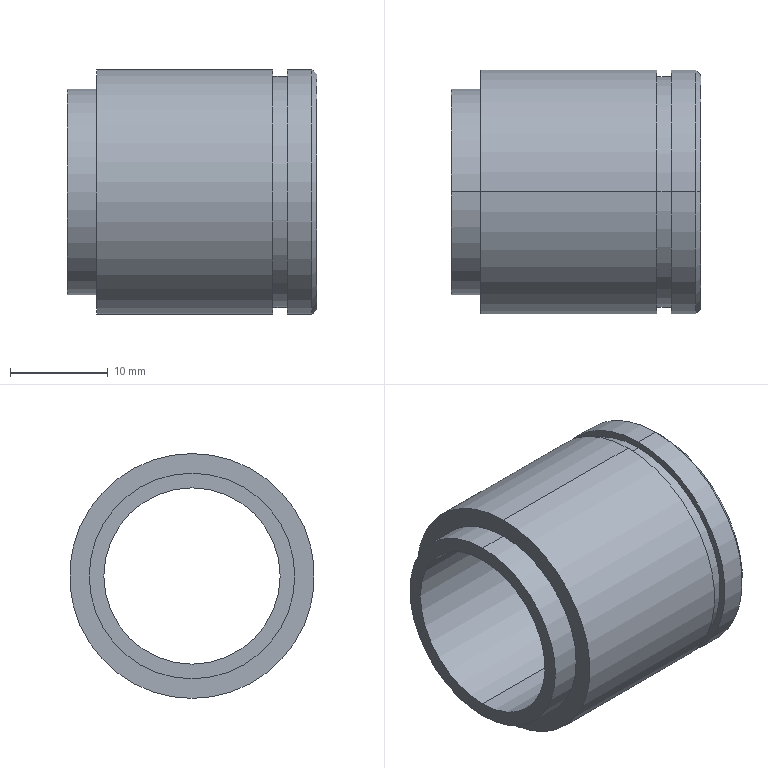Part | STEP file | 1 solid | 19 faces | box 25.5 x 25 x 25 mm | volume 5476 mm3 | cylinder 10 | plane 5 | cone 4 | commonest cylinder face diameters 25 x4 18 x2 21 x2 23.6 x2
STEP:
#1=CARTESIAN_POINT('',(0.,0.,0.));
#2=DIRECTION('',(0.,0.,1.));
#3=DIRECTION('',(1.,0.,0.));
#4=AXIS2_PLACEMENT_3D('',#1,#2,#3);
#5=CARTESIAN_POINT('',(3.,0.,-12.5));
#6=VERTEX_POINT('',#5);
#7=CARTESIAN_POINT('',(3.,0.,12.5));
#8=VERTEX_POINT('',#7);
#9=CARTESIAN_POINT('',(3.,0.,0.));
#10=DIRECTION('',(1.,0.,0.));
#11=DIRECTION('',(0.,0.,-1.));
#12=AXIS2_PLACEMENT_3D('',#9,#10,#11);
#13=CIRCLE('',#12,12.5);
#14=CARTESIAN_POINT('',(12.,0.,0.));
#15=DIRECTION('',(1.,0.,0.));
#16=DIRECTION('',(0.,0.,-1.));
#17=AXIS2_PLACEMENT_3D('',#14,#15,#16);
#18=CYLINDRICAL_SURFACE('',#17,12.5);
#19=CARTESIAN_POINT('',(0.,-9.));
#20=DIRECTION('',(1.,0.));
#21=VECTOR('',#20,1.);
#22=LINE('',#19,#21);
#23=(GEOMETRIC_REPRESENTATION_CONTEXT(2)PARAMETRIC_REPRESENTATION_CONTEXT()REPRESENTATION_CONTEXT('',''));
#24=DEFINITIONAL_REPRESENTATION('',(#22),#23);
#25=PCURVE('',#18,#24);
#26=CARTESIAN_POINT('',(3.,11.5,0.));
#27=DIRECTION('',(-1.,0.,0.));
#28=DIRECTION('',(0.,0.,1.));
#29=AXIS2_PLACEMENT_3D('',#26,#27,#28);
#30=PLANE('',#29);
#31=CARTESIAN_POINT('',(-12.5,-11.5));
#32=CARTESIAN_POINT('',(-12.5,10.151));
#33=CARTESIAN_POINT('',(6.25,-0.6747));
#34=CARTESIAN_POINT('',(25.,-11.5));
#35=CARTESIAN_POINT('',(6.25,-22.325));
#36=CARTESIAN_POINT('',(-12.5,-33.151));
#37=CARTESIAN_POINT('',(-12.5,-11.5));
#38=(BOUNDED_CURVE()B_SPLINE_CURVE(2,(#31,#32,#33,#34,#35,#36,#37),.UNSPECIFIED.,.T.,.F.)B_SPLINE_CURVE_WITH_KNOTS((1,2,2,2,2,1),(-2.094,0.,2.094,4.189,6.283,8.378),.UNSPECIFIED.)CURVE()GEOMETRIC_REPRESENTATION_ITEM()RATIONAL_B_SPLINE_CURVE((1.,0.5,1.,0.5,1.,0.5,1.))REPRESENTATION_ITEM(''));
#39=(GEOMETRIC_REPRESENTATION_CONTEXT(2)PARAMETRIC_REPRESENTATION_CONTEXT()REPRESENTATION_CONTEXT('',''));
#40=DEFINITIONAL_REPRESENTATION('',(#38),#39);
#41=PCURVE('',#30,#40);
#42=SURFACE_CURVE('',#13,(#25,#41),.PCURVE_S1.);
#43=EDGE_CURVE('',#6,#8,#42,.T.);
#44=ORIENTED_EDGE('',*,*,#43,.T.);
#45=CARTESIAN_POINT('',(21.,0.,12.5));
#46=VERTEX_POINT('',#45);
#47=CARTESIAN_POINT('',(12.,0.,12.5));
#48=DIRECTION('',(1.,0.,0.));
#49=VECTOR('',#48,1.);
#50=LINE('',#47,#49);
#51=CARTESIAN_POINT('',(3.142,0.));
#52=DIRECTION('',(0.,1.));
#53=VECTOR('',#52,1.);
#54=LINE('',#51,#53);
#55=(GEOMETRIC_REPRESENTATION_CONTEXT(2)PARAMETRIC_REPRESENTATION_CONTEXT()REPRESENTATION_CONTEXT('',''));
#56=DEFINITIONAL_REPRESENTATION('',(#54),#55);
#57=PCURVE('',#18,#56);
#58=CARTESIAN_POINT('',(12.,0.,0.));
#59=DIRECTION('',(1.,0.,0.));
#60=DIRECTION('',(0.,0.,-1.));
#61=AXIS2_PLACEMENT_3D('',#58,#59,#60);
#62=CYLINDRICAL_SURFACE('',#61,12.5);
#63=CARTESIAN_POINT('',(3.142,0.));
#64=DIRECTION('',(0.,1.));
#65=VECTOR('',#64,1.);
#66=LINE('',#63,#65);
#67=(GEOMETRIC_REPRESENTATION_CONTEXT(2)PARAMETRIC_REPRESENTATION_CONTEXT()REPRESENTATION_CONTEXT('',''));
#68=DEFINITIONAL_REPRESENTATION('',(#66),#67);
#69=PCURVE('',#62,#68);
#70=SURFACE_CURVE('',#50,(#57,#69),.PCURVE_S1.);
#71=EDGE_CURVE('',#8,#46,#70,.T.);
#72=ORIENTED_EDGE('',*,*,#71,.T.);
#73=CARTESIAN_POINT('',(21.,0.,-12.5));
#74=VERTEX_POINT('',#73);
#75=CARTESIAN_POINT('',(21.,0.,0.));
#76=DIRECTION('',(-1.,0.,0.));
#77=DIRECTION('',(0.,0.,-1.));
#78=AXIS2_PLACEMENT_3D('',#75,#76,#77);
#79=CIRCLE('',#78,12.5);
#80=CARTESIAN_POINT('',(6.283,9.));
#81=DIRECTION('',(-1.,0.));
#82=VECTOR('',#81,1.);
#83=LINE('',#80,#82);
#84=(GEOMETRIC_REPRESENTATION_CONTEXT(2)PARAMETRIC_REPRESENTATION_CONTEXT()REPRESENTATION_CONTEXT('',''));
#85=DEFINITIONAL_REPRESENTATION('',(#83),#84);
#86=PCURVE('',#18,#85);
#87=CARTESIAN_POINT('',(21.,12.15,0.));
#88=DIRECTION('',(1.,0.,0.));
#89=DIRECTION('',(0.,0.,-1.));
#90=AXIS2_PLACEMENT_3D('',#87,#88,#89);
#91=PLANE('',#90);
#92=CARTESIAN_POINT('',(12.5,-12.15));
#93=CARTESIAN_POINT('',(12.5,-33.801));
#94=CARTESIAN_POINT('',(-6.25,-22.975));
#95=CARTESIAN_POINT('',(-25.,-12.15));
#96=CARTESIAN_POINT('',(-6.25,-1.325));
#97=CARTESIAN_POINT('',(12.5,9.501));
#98=CARTESIAN_POINT('',(12.5,-12.15));
#99=(BOUNDED_CURVE()B_SPLINE_CURVE(2,(#92,#93,#94,#95,#96,#97,#98),.UNSPECIFIED.,.T.,.F.)B_SPLINE_CURVE_WITH_KNOTS((1,2,2,2,2,1),(-2.094,0.,2.094,4.189,6.283,8.378),.UNSPECIFIED.)CURVE()GEOMETRIC_REPRESENTATION_ITEM()RATIONAL_B_SPLINE_CURVE((1.,0.5,1.,0.5,1.,0.5,1.))REPRESENTATION_ITEM(''));
#100=(GEOMETRIC_REPRESENTATION_CONTEXT(2)PARAMETRIC_REPRESENTATION_CONTEXT()REPRESENTATION_CONTEXT('',''));
#101=DEFINITIONAL_REPRESENTATION('',(#99),#100);
#102=PCURVE('',#91,#101);
#103=SURFACE_CURVE('',#79,(#86,#102),.PCURVE_S1.);
#104=EDGE_CURVE('',#46,#74,#103,.T.);
#105=ORIENTED_EDGE('',*,*,#104,.T.);
#106=CARTESIAN_POINT('',(12.,0.,-12.5));
#107=DIRECTION('',(1.,0.,0.));
#108=VECTOR('',#107,1.);
#109=LINE('',#106,#108);
#110=CARTESIAN_POINT('',(0.,0.));
#111=DIRECTION('',(0.,1.));
#112=VECTOR('',#111,1.);
#113=LINE('',#110,#112);
#114=(GEOMETRIC_REPRESENTATION_CONTEXT(2)PARAMETRIC_REPRESENTATION_CONTEXT()REPRESENTATION_CONTEXT('',''));
#115=DEFINITIONAL_REPRESENTATION('',(#113),#114);
#116=PCURVE('',#18,#115);
#117=CARTESIAN_POINT('',(6.283,0.));
#118=DIRECTION('',(0.,1.));
#119=VECTOR('',#118,1.);
#120=LINE('',#117,#119);
#121=(GEOMETRIC_REPRESENTATION_CONTEXT(2)PARAMETRIC_REPRESENTATION_CONTEXT()REPRESENTATION_CONTEXT('',''));
#122=DEFINITIONAL_REPRESENTATION('',(#120),#121);
#123=PCURVE('',#62,#122);
#124=SURFACE_CURVE('',#109,(#116,#123),.PCURVE_S1.);
#125=EDGE_CURVE('',#6,#74,#124,.T.);
#126=ORIENTED_EDGE('',*,*,#125,.F.);
#127=EDGE_LOOP('',(#44,#72,#105,#126));
#128=FACE_BOUND('',#127,.T.);
#129=ADVANCED_FACE('',(#128),#18,.T.);
#130=CARTESIAN_POINT('',(0.,0.,-10.5));
#131=VERTEX_POINT('',#130);
#132=CARTESIAN_POINT('',(0.,0.,10.5));
#133=VERTEX_POINT('',#132);
#134=CARTESIAN_POINT('',(0.,0.,0.));
#135=DIRECTION('',(1.,0.,0.));
#136=DIRECTION('',(0.,0.,-1.));
#137=AXIS2_PLACEMENT_3D('',#134,#135,#136);
#138=CIRCLE('',#137,10.5);
#139=CARTESIAN_POINT('',(1.5,0.,0.));
#140=DIRECTION('',(1.,0.,0.));
#141=DIRECTION('',(0.,0.,-1.));
#142=AXIS2_PLACEMENT_3D('',#139,#140,#141);
#143=CYLINDRICAL_SURFACE('',#142,10.5);
#144=CARTESIAN_POINT('',(0.,-1.5));
#145=DIRECTION('',(1.,0.));
#146=VECTOR('',#145,1.);
#147=LINE('',#144,#146);
#148=(GEOMETRIC_REPRESENTATION_CONTEXT(2)PARAMETRIC_REPRESENTATION_CONTEXT()REPRESENTATION_CONTEXT('',''));
#149=DEFINITIONAL_REPRESENTATION('',(#147),#148);
#150=PCURVE('',#143,#149);
#151=CARTESIAN_POINT('',(0.,9.75,0.));
#152=DIRECTION('',(-1.,0.,0.));
#153=DIRECTION('',(0.,0.,1.));
#154=AXIS2_PLACEMENT_3D('',#151,#152,#153);
#155=PLANE('',#154);
#156=CARTESIAN_POINT('',(-10.5,-9.75));
#157=CARTESIAN_POINT('',(-10.5,8.437));
#158=CARTESIAN_POINT('',(5.25,-0.6567));
#159=CARTESIAN_POINT('',(21.,-9.75));
#160=CARTESIAN_POINT('',(5.25,-18.843));
#161=CARTESIAN_POINT('',(-10.5,-27.937));
#162=CARTESIAN_POINT('',(-10.5,-9.75));
#163=(BOUNDED_CURVE()B_SPLINE_CURVE(2,(#156,#157,#158,#159,#160,#161,#162),.UNSPECIFIED.,.T.,.F.)B_SPLINE_CURVE_WITH_KNOTS((1,2,2,2,2,1),(-2.094,0.,2.094,4.189,6.283,8.378),.UNSPECIFIED.)CURVE()GEOMETRIC_REPRESENTATION_ITEM()RATIONAL_B_SPLINE_CURVE((1.,0.5,1.,0.5,1.,0.5,1.))REPRESENTATION_ITEM(''));
#164=(GEOMETRIC_REPRESENTATION_CONTEXT(2)PARAMETRIC_REPRESENTATION_CONTEXT()REPRESENTATION_CONTEXT('',''));
#165=DEFINITIONAL_REPRESENTATION('',(#163),#164);
#166=PCURVE('',#155,#165);
#167=SURFACE_CURVE('',#138,(#150,#166),.PCURVE_S1.);
#168=EDGE_CURVE('',#131,#133,#167,.T.);
#169=ORIENTED_EDGE('',*,*,#168,.T.);
#170=CARTESIAN_POINT('',(3.,0.,10.5));
#171=VERTEX_POINT('',#170);
#172=CARTESIAN_POINT('',(1.5,0.,10.5));
#173=DIRECTION('',(1.,0.,0.));
#174=VECTOR('',#173,1.);
#175=LINE('',#172,#174);
#176=CARTESIAN_POINT('',(3.142,0.));
#177=DIRECTION('',(0.,1.));
#178=VECTOR('',#177,1.);
#179=LINE('',#176,#178);
#180=(GEOMETRIC_REPRESENTATION_CONTEXT(2)PARAMETRIC_REPRESENTATION_CONTEXT()REPRESENTATION_CONTEXT('',''));
#181=DEFINITIONAL_REPRESENTATION('',(#179),#180);
#182=PCURVE('',#143,#181);
#183=CARTESIAN_POINT('',(1.5,0.,0.));
#184=DIRECTION('',(1.,0.,0.));
#185=DIRECTION('',(0.,0.,-1.));
#186=AXIS2_PLACEMENT_3D('',#183,#184,#185);
#187=CYLINDRICAL_SURFACE('',#186,10.5);
#188=CARTESIAN_POINT('',(3.142,0.));
#189=DIRECTION('',(0.,1.));
#190=VECTOR('',#189,1.);
#191=LINE('',#188,#190);
#192=(GEOMETRIC_REPRESENTATION_CONTEXT(2)PARAMETRIC_REPRESENTATION_CONTEXT()REPRESENTATION_CONTEXT('',''));
#193=DEFINITIONAL_REPRESENTATION('',(#191),#192);
#194=PCURVE('',#187,#193);
#195=SURFACE_CURVE('',#175,(#182,#194),.PCURVE_S1.);
#196=EDGE_CURVE('',#133,#171,#195,.T.);
#197=ORIENTED_EDGE('',*,*,#196,.T.);
#198=CARTESIAN_POINT('',(3.,0.,-10.5));
#199=VERTEX_POINT('',#198);
#200=CARTESIAN_POINT('',(3.,0.,0.));
#201=DIRECTION('',(1.,0.,0.));
#202=DIRECTION('',(0.,0.,-1.));
#203=AXIS2_PLACEMENT_3D('',#200,#201,#202);
#204=CIRCLE('',#203,10.5);
#205=CARTESIAN_POINT('',(0.,1.5));
#206=DIRECTION('',(1.,0.));
#207=VECTOR('',#206,1.);
#208=LINE('',#205,#207);
#209=(GEOMETRIC_REPRESENTATION_CONTEXT(2)PARAMETRIC_REPRESENTATION_CONTEXT()REPRESENTATION_CONTEXT('',''));
#210=DEFINITIONAL_REPRESENTATION('',(#208),#209);
#211=PCURVE('',#143,#210);
#212=CARTESIAN_POINT('',(-10.5,-11.5));
#213=CARTESIAN_POINT('',(-10.5,6.687));
#214=CARTESIAN_POINT('',(5.25,-2.407));
#215=CARTESIAN_POINT('',(21.,-11.5));
#216=CARTESIAN_POINT('',(5.25,-20.593));
#217=CARTESIAN_POINT('',(-10.5,-29.687));
#218=CARTESIAN_POINT('',(-10.5,-11.5));
#219=(BOUNDED_CURVE()B_SPLINE_CURVE(2,(#212,#213,#214,#215,#216,#217,#218),.UNSPECIFIED.,.T.,.F.)B_SPLINE_CURVE_WITH_KNOTS((1,2,2,2,2,1),(-2.094,0.,2.094,4.189,6.283,8.378),.UNSPECIFIED.)CURVE()GEOMETRIC_REPRESENTATION_ITEM()RATIONAL_B_SPLINE_CURVE((1.,0.5,1.,0.5,1.,0.5,1.))REPRESENTATION_ITEM(''));
#220=(GEOMETRIC_REPRESENTATION_CONTEXT(2)PARAMETRIC_REPRESENTATION_CONTEXT()REPRESENTATION_CONTEXT('',''));
#221=DEFINITIONAL_REPRESENTATION('',(#219),#220);
#222=PCURVE('',#30,#221);
#223=SURFACE_CURVE('',#204,(#211,#222),.PCURVE_S1.);
#224=EDGE_CURVE('',#199,#171,#223,.T.);
#225=ORIENTED_EDGE('',*,*,#224,.F.);
#226=CARTESIAN_POINT('',(1.5,0.,-10.5));
#227=DIRECTION('',(1.,0.,0.));
#228=VECTOR('',#227,1.);
#229=LINE('',#226,#228);
#230=CARTESIAN_POINT('',(0.,0.));
#231=DIRECTION('',(0.,1.));
#232=VECTOR('',#231,1.);
#233=LINE('',#230,#232);
#234=(GEOMETRIC_REPRESENTATION_CONTEXT(2)PARAMETRIC_REPRESENTATION_CONTEXT()REPRESENTATION_CONTEXT('',''));
#235=DEFINITIONAL_REPRESENTATION('',(#233),#234);
#236=PCURVE('',#143,#235);
#237=CARTESIAN_POINT('',(6.283,0.));
#238=DIRECTION('',(0.,1.));
#239=VECTOR('',#238,1.);
#240=LINE('',#237,#239);
#241=(GEOMETRIC_REPRESENTATION_CONTEXT(2)PARAMETRIC_REPRESENTATION_CONTEXT()REPRESENTATION_CONTEXT('',''));
#242=DEFINITIONAL_REPRESENTATION('',(#240),#241);
#243=PCURVE('',#187,#242);
#244=SURFACE_CURVE('',#229,(#236,#243),.PCURVE_S1.);
#245=EDGE_CURVE('',#131,#199,#244,.T.);
#246=ORIENTED_EDGE('',*,*,#245,.F.);
#247=EDGE_LOOP('',(#169,#197,#225,#246));
#248=FACE_BOUND('',#247,.T.);
#249=ADVANCED_FACE('',(#248),#143,.T.);
#250=CARTESIAN_POINT('',(21.,0.,11.8));
#251=VERTEX_POINT('',#250);
#252=CARTESIAN_POINT('',(21.,0.,-11.8));
#253=VERTEX_POINT('',#252);
#254=CARTESIAN_POINT('',(21.,0.,0.));
#255=DIRECTION('',(-1.,0.,0.));
#256=DIRECTION('',(0.,0.,-1.));
#257=AXIS2_PLACEMENT_3D('',#254,#255,#256);
#258=CIRCLE('',#257,11.8);
#259=CARTESIAN_POINT('',(21.75,0.,0.));
#260=DIRECTION('',(1.,0.,0.));
#261=DIRECTION('',(0.,0.,-1.));
#262=AXIS2_PLACEMENT_3D('',#259,#260,#261);
#263=CYLINDRICAL_SURFACE('',#262,11.8);
#264=CARTESIAN_POINT('',(6.283,-0.75));
#265=DIRECTION('',(-1.,0.));
#266=VECTOR('',#265,1.);
#267=LINE('',#264,#266);
#268=(GEOMETRIC_REPRESENTATION_CONTEXT(2)PARAMETRIC_REPRESENTATION_CONTEXT()REPRESENTATION_CONTEXT('',''));
#269=DEFINITIONAL_REPRESENTATION('',(#267),#268);
#270=PCURVE('',#263,#269);
#271=CARTESIAN_POINT('',(11.8,-12.15));
#272=CARTESIAN_POINT('',(11.8,-32.588));
#273=CARTESIAN_POINT('',(-5.9,-22.369));
#274=CARTESIAN_POINT('',(-23.6,-12.15));
#275=CARTESIAN_POINT('',(-5.9,-1.931));
#276=CARTESIAN_POINT('',(11.8,8.288));
#277=CARTESIAN_POINT('',(11.8,-12.15));
#278=(BOUNDED_CURVE()B_SPLINE_CURVE(2,(#271,#272,#273,#274,#275,#276,#277),.UNSPECIFIED.,.T.,.F.)B_SPLINE_CURVE_WITH_KNOTS((1,2,2,2,2,1),(-2.094,0.,2.094,4.189,6.283,8.378),.UNSPECIFIED.)CURVE()GEOMETRIC_REPRESENTATION_ITEM()RATIONAL_B_SPLINE_CURVE((1.,0.5,1.,0.5,1.,0.5,1.))REPRESENTATION_ITEM(''));
#279=(GEOMETRIC_REPRESENTATION_CONTEXT(2)PARAMETRIC_REPRESENTATION_CONTEXT()REPRESENTATION_CONTEXT('',''));
#280=DEFINITIONAL_REPRESENTATION('',(#278),#279);
#281=PCURVE('',#91,#280);
#282=SURFACE_CURVE('',#258,(#270,#281),.PCURVE_S1.);
#283=EDGE_CURVE('',#251,#253,#282,.T.);
#284=ORIENTED_EDGE('',*,*,#283,.F.);
#285=CARTESIAN_POINT('',(22.5,0.,11.8));
#286=VERTEX_POINT('',#285);
#287=CARTESIAN_POINT('',(21.75,0.,11.8));
#288=DIRECTION('',(1.,0.,0.));
#289=VECTOR('',#288,1.);
#290=LINE('',#287,#289);
#291=CARTESIAN_POINT('',(3.142,0.));
#292=DIRECTION('',(0.,1.));
#293=VECTOR('',#292,1.);
#294=LINE('',#291,#293);
#295=(GEOMETRIC_REPRESENTATION_CONTEXT(2)PARAMETRIC_REPRESENTATION_CONTEXT()REPRESENTATION_CONTEXT('',''));
#296=DEFINITIONAL_REPRESENTATION('',(#294),#295);
#297=PCURVE('',#263,#296);
#298=CARTESIAN_POINT('',(21.75,0.,0.));
#299=DIRECTION('',(1.,0.,0.));
#300=DIRECTION('',(0.,0.,-1.));
#301=AXIS2_PLACEMENT_3D('',#298,#299,#300);
#302=CYLINDRICAL_SURFACE('',#301,11.8);
#303=CARTESIAN_POINT('',(3.142,0.));
#304=DIRECTION('',(0.,1.));
#305=VECTOR('',#304,1.);
#306=LINE('',#303,#305);
#307=(GEOMETRIC_REPRESENTATION_CONTEXT(2)PARAMETRIC_REPRESENTATION_CONTEXT()REPRESENTATION_CONTEXT('',''));
#308=DEFINITIONAL_REPRESENTATION('',(#306),#307);
#309=PCURVE('',#302,#308);
#310=SURFACE_CURVE('',#290,(#297,#309),.PCURVE_S1.);
#311=EDGE_CURVE('',#251,#286,#310,.T.);
#312=ORIENTED_EDGE('',*,*,#311,.T.);
#313=CARTESIAN_POINT('',(22.5,0.,-11.8));
#314=VERTEX_POINT('',#313);
#315=CARTESIAN_POINT('',(22.5,0.,0.));
#316=DIRECTION('',(-1.,0.,0.));
#317=DIRECTION('',(0.,0.,-1.));
#318=AXIS2_PLACEMENT_3D('',#315,#316,#317);
#319=CIRCLE('',#318,11.8);
#320=CARTESIAN_POINT('',(6.283,0.75));
#321=DIRECTION('',(-1.,0.));
#322=VECTOR('',#321,1.);
#323=LINE('',#320,#322);
#324=(GEOMETRIC_REPRESENTATION_CONTEXT(2)PARAMETRIC_REPRESENTATION_CONTEXT()REPRESENTATION_CONTEXT('',''));
#325=DEFINITIONAL_REPRESENTATION('',(#323),#324);
#326=PCURVE('',#263,#325);
#327=CARTESIAN_POINT('',(22.5,12.15,0.));
#328=DIRECTION('',(-1.,0.,0.));
#329=DIRECTION('',(0.,0.,1.));
#330=AXIS2_PLACEMENT_3D('',#327,#328,#329);
#331=PLANE('',#330);
#332=CARTESIAN_POINT('',(0.,-12.15));
#333=DIRECTION('',(-1.,0.));
#334=AXIS2_PLACEMENT_2D('',#332,#333);
#335=CIRCLE('',#334,11.8);
#336=(GEOMETRIC_REPRESENTATION_CONTEXT(2)PARAMETRIC_REPRESENTATION_CONTEXT()REPRESENTATION_CONTEXT('',''));
#337=DEFINITIONAL_REPRESENTATION('',(#335),#336);
#338=PCURVE('',#331,#337);
#339=SURFACE_CURVE('',#319,(#326,#338),.PCURVE_S1.);
#340=EDGE_CURVE('',#286,#314,#339,.T.);
#341=ORIENTED_EDGE('',*,*,#340,.T.);
#342=CARTESIAN_POINT('',(21.75,0.,-11.8));
#343=DIRECTION('',(1.,0.,0.));
#344=VECTOR('',#343,1.);
#345=LINE('',#342,#344);
#346=CARTESIAN_POINT('',(0.,0.));
#347=DIRECTION('',(0.,1.));
#348=VECTOR('',#347,1.);
#349=LINE('',#346,#348);
#350=(GEOMETRIC_REPRESENTATION_CONTEXT(2)PARAMETRIC_REPRESENTATION_CONTEXT()REPRESENTATION_CONTEXT('',''));
#351=DEFINITIONAL_REPRESENTATION('',(#349),#350);
#352=PCURVE('',#263,#351);
#353=CARTESIAN_POINT('',(6.283,0.));
#354=DIRECTION('',(0.,1.));
#355=VECTOR('',#354,1.);
#356=LINE('',#353,#355);
#357=(GEOMETRIC_REPRESENTATION_CONTEXT(2)PARAMETRIC_REPRESENTATION_CONTEXT()REPRESENTATION_CONTEXT('',''));
#358=DEFINITIONAL_REPRESENTATION('',(#356),#357);
#359=PCURVE('',#302,#358);
#360=SURFACE_CURVE('',#345,(#352,#359),.PCURVE_S1.);
#361=EDGE_CURVE('',#253,#314,#360,.T.);
#362=ORIENTED_EDGE('',*,*,#361,.F.);
#363=EDGE_LOOP('',(#284,#312,#341,#362));
#364=FACE_BOUND('',#363,.T.);
#365=ADVANCED_FACE('',(#364),#263,.T.);
#366=CARTESIAN_POINT('',(0.,0.,-9.));
#367=VERTEX_POINT('',#366);
#368=CARTESIAN_POINT('',(24.5,0.,-9.));
#369=VERTEX_POINT('',#368);
#370=CARTESIAN_POINT('',(12.25,0.,-9.));
#371=DIRECTION('',(1.,0.,0.));
#372=VECTOR('',#371,1.);
#373=LINE('',#370,#372);
#374=CARTESIAN_POINT('',(12.25,0.,0.));
#375=DIRECTION('',(1.,0.,0.));
#376=DIRECTION('',(0.,0.,-1.));
#377=AXIS2_PLACEMENT_3D('',#374,#375,#376);
#378=CYLINDRICAL_SURFACE('',#377,9.);
#379=CARTESIAN_POINT('',(6.283,0.));
#380=DIRECTION('',(0.,1.));
#381=VECTOR('',#380,1.);
#382=LINE('',#379,#381);
#383=(GEOMETRIC_REPRESENTATION_CONTEXT(2)PARAMETRIC_REPRESENTATION_CONTEXT()REPRESENTATION_CONTEXT('',''));
#384=DEFINITIONAL_REPRESENTATION('',(#382),#383);
#385=PCURVE('',#378,#384);
#386=CARTESIAN_POINT('',(12.25,0.,0.));
#387=DIRECTION('',(1.,0.,0.));
#388=DIRECTION('',(0.,0.,-1.));
#389=AXIS2_PLACEMENT_3D('',#386,#387,#388);
#390=CYLINDRICAL_SURFACE('',#389,9.);
#391=CARTESIAN_POINT('',(0.,0.));
#392=DIRECTION('',(0.,1.));
#393=VECTOR('',#392,1.);
#394=LINE('',#391,#393);
#395=(GEOMETRIC_REPRESENTATION_CONTEXT(2)PARAMETRIC_REPRESENTATION_CONTEXT()REPRESENTATION_CONTEXT('',''));
#396=DEFINITIONAL_REPRESENTATION('',(#394),#395);
#397=PCURVE('',#390,#396);
#398=SURFACE_CURVE('',#373,(#385,#397),.PCURVE_S1.);
#399=EDGE_CURVE('',#367,#369,#398,.T.);
#400=ORIENTED_EDGE('',*,*,#399,.T.);
#401=CARTESIAN_POINT('',(24.5,0.,9.));
#402=VERTEX_POINT('',#401);
#403=CARTESIAN_POINT('',(24.5,0.,0.));
#404=DIRECTION('',(-1.,0.,0.));
#405=DIRECTION('',(0.,0.,-1.));
#406=AXIS2_PLACEMENT_3D('',#403,#404,#405);
#407=CIRCLE('',#406,9.);
#408=CARTESIAN_POINT('',(6.283,12.25));
#409=DIRECTION('',(-1.,0.));
#410=VECTOR('',#409,1.);
#411=LINE('',#408,#410);
#412=(GEOMETRIC_REPRESENTATION_CONTEXT(2)PARAMETRIC_REPRESENTATION_CONTEXT()REPRESENTATION_CONTEXT('',''));
#413=DEFINITIONAL_REPRESENTATION('',(#411),#412);
#414=PCURVE('',#378,#413);
#415=CARTESIAN_POINT('',(25.5,0.,0.));
#416=DIRECTION('',(1.,0.,0.));
#417=DIRECTION('',(0.,0.,-1.));
#418=AXIS2_PLACEMENT_3D('',#415,#416,#417);
#419=CONICAL_SURFACE('',#418,10.,0.7854);
#420=CARTESIAN_POINT('',(6.283,-1.));
#421=DIRECTION('',(-1.,0.));
#422=VECTOR('',#421,1.);
#423=LINE('',#420,#422);
#424=(GEOMETRIC_REPRESENTATION_CONTEXT(2)PARAMETRIC_REPRESENTATION_CONTEXT()REPRESENTATION_CONTEXT('',''));
#425=DEFINITIONAL_REPRESENTATION('',(#423),#424);
#426=PCURVE('',#419,#425);
#427=SURFACE_CURVE('',#407,(#414,#426),.PCURVE_S1.);
#428=EDGE_CURVE('',#369,#402,#427,.T.);
#429=ORIENTED_EDGE('',*,*,#428,.T.);
#430=CARTESIAN_POINT('',(0.,0.,9.));
#431=VERTEX_POINT('',#430);
#432=CARTESIAN_POINT('',(12.25,0.,9.));
#433=DIRECTION('',(1.,0.,0.));
#434=VECTOR('',#433,1.);
#435=LINE('',#432,#434);
#436=CARTESIAN_POINT('',(3.142,0.));
#437=DIRECTION('',(0.,1.));
#438=VECTOR('',#437,1.);
#439=LINE('',#436,#438);
#440=(GEOMETRIC_REPRESENTATION_CONTEXT(2)PARAMETRIC_REPRESENTATION_CONTEXT()REPRESENTATION_CONTEXT('',''));
#441=DEFINITIONAL_REPRESENTATION('',(#439),#440);
#442=PCURVE('',#378,#441);
#443=CARTESIAN_POINT('',(3.142,0.));
#444=DIRECTION('',(0.,1.));
#445=VECTOR('',#444,1.);
#446=LINE('',#443,#445);
#447=(GEOMETRIC_REPRESENTATION_CONTEXT(2)PARAMETRIC_REPRESENTATION_CONTEXT()REPRESENTATION_CONTEXT('',''));
#448=DEFINITIONAL_REPRESENTATION('',(#446),#447);
#449=PCURVE('',#390,#448);
#450=SURFACE_CURVE('',#435,(#442,#449),.PCURVE_S1.);
#451=EDGE_CURVE('',#431,#402,#450,.T.);
#452=ORIENTED_EDGE('',*,*,#451,.F.);
#453=CARTESIAN_POINT('',(0.,0.,0.));
#454=DIRECTION('',(1.,0.,0.));
#455=DIRECTION('',(0.,0.,-1.));
#456=AXIS2_PLACEMENT_3D('',#453,#454,#455);
#457=CIRCLE('',#456,9.);
#458=CARTESIAN_POINT('',(0.,-12.25));
#459=DIRECTION('',(1.,0.));
#460=VECTOR('',#459,1.);
#461=LINE('',#458,#460);
#462=(GEOMETRIC_REPRESENTATION_CONTEXT(2)PARAMETRIC_REPRESENTATION_CONTEXT()REPRESENTATION_CONTEXT('',''));
#463=DEFINITIONAL_REPRESENTATION('',(#461),#462);
#464=PCURVE('',#378,#463);
#465=CARTESIAN_POINT('',(-9.,-9.75));
#466=CARTESIAN_POINT('',(-9.,5.838));
#467=CARTESIAN_POINT('',(4.5,-1.956));
#468=CARTESIAN_POINT('',(18.,-9.75));
#469=CARTESIAN_POINT('',(4.5,-17.544));
#470=CARTESIAN_POINT('',(-9.,-25.338));
#471=CARTESIAN_POINT('',(-9.,-9.75));
#472=(BOUNDED_CURVE()B_SPLINE_CURVE(2,(#465,#466,#467,#468,#469,#470,#471),.UNSPECIFIED.,.T.,.F.)B_SPLINE_CURVE_WITH_KNOTS((1,2,2,2,2,1),(-2.094,0.,2.094,4.189,6.283,8.378),.UNSPECIFIED.)CURVE()GEOMETRIC_REPRESENTATION_ITEM()RATIONAL_B_SPLINE_CURVE((1.,0.5,1.,0.5,1.,0.5,1.))REPRESENTATION_ITEM(''));
#473=(GEOMETRIC_REPRESENTATION_CONTEXT(2)PARAMETRIC_REPRESENTATION_CONTEXT()REPRESENTATION_CONTEXT('',''));
#474=DEFINITIONAL_REPRESENTATION('',(#472),#473);
#475=PCURVE('',#155,#474);
#476=SURFACE_CURVE('',#457,(#464,#475),.PCURVE_S1.);
#477=EDGE_CURVE('',#431,#367,#476,.T.);
#478=ORIENTED_EDGE('',*,*,#477,.T.);
#479=EDGE_LOOP('',(#400,#429,#452,#478));
#480=FACE_BOUND('',#479,.F.);
#481=ADVANCED_FACE('',(#480),#378,.F.);
#482=CARTESIAN_POINT('',(22.5,0.,12.5));
#483=VERTEX_POINT('',#482);
#484=CARTESIAN_POINT('',(22.5,0.,-12.5));
#485=VERTEX_POINT('',#484);
#486=CARTESIAN_POINT('',(22.5,0.,0.));
#487=DIRECTION('',(-1.,0.,0.));
#488=DIRECTION('',(0.,0.,-1.));
#489=AXIS2_PLACEMENT_3D('',#486,#487,#488);
#490=CIRCLE('',#489,12.5);
#491=CARTESIAN_POINT('',(23.75,0.,0.));
#492=DIRECTION('',(1.,0.,0.));
#493=DIRECTION('',(0.,0.,-1.));
#494=AXIS2_PLACEMENT_3D('',#491,#492,#493);
#495=CYLINDRICAL_SURFACE('',#494,12.5);
#496=CARTESIAN_POINT('',(6.283,-1.25));
#497=DIRECTION('',(-1.,0.));
#498=VECTOR('',#497,1.);
#499=LINE('',#496,#498);
#500=(GEOMETRIC_REPRESENTATION_CONTEXT(2)PARAMETRIC_REPRESENTATION_CONTEXT()REPRESENTATION_CONTEXT('',''));
#501=DEFINITIONAL_REPRESENTATION('',(#499),#500);
#502=PCURVE('',#495,#501);
#503=CARTESIAN_POINT('',(0.,-12.15));
#504=DIRECTION('',(-1.,0.));
#505=AXIS2_PLACEMENT_2D('',#503,#504);
#506=CIRCLE('',#505,12.5);
#507=(GEOMETRIC_REPRESENTATION_CONTEXT(2)PARAMETRIC_REPRESENTATION_CONTEXT()REPRESENTATION_CONTEXT('',''));
#508=DEFINITIONAL_REPRESENTATION('',(#506),#507);
#509=PCURVE('',#331,#508);
#510=SURFACE_CURVE('',#490,(#502,#509),.PCURVE_S1.);
#511=EDGE_CURVE('',#483,#485,#510,.T.);
#512=ORIENTED_EDGE('',*,*,#511,.F.);
#513=CARTESIAN_POINT('',(25.,0.,12.5));
#514=VERTEX_POINT('',#513);
#515=CARTESIAN_POINT('',(23.75,0.,12.5));
#516=DIRECTION('',(1.,0.,0.));
#517=VECTOR('',#516,1.);
#518=LINE('',#515,#517);
#519=CARTESIAN_POINT('',(3.142,0.));
#520=DIRECTION('',(0.,1.));
#521=VECTOR('',#520,1.);
#522=LINE('',#519,#521);
#523=(GEOMETRIC_REPRESENTATION_CONTEXT(2)PARAMETRIC_REPRESENTATION_CONTEXT()REPRESENTATION_CONTEXT('',''));
#524=DEFINITIONAL_REPRESENTATION('',(#522),#523);
#525=PCURVE('',#495,#524);
#526=CARTESIAN_POINT('',(23.75,0.,0.));
#527=DIRECTION('',(1.,0.,0.));
#528=DIRECTION('',(0.,0.,-1.));
#529=AXIS2_PLACEMENT_3D('',#526,#527,#528);
#530=CYLINDRICAL_SURFACE('',#529,12.5);
#531=CARTESIAN_POINT('',(3.142,0.));
#532=DIRECTION('',(0.,1.));
#533=VECTOR('',#532,1.);
#534=LINE('',#531,#533);
#535=(GEOMETRIC_REPRESENTATION_CONTEXT(2)PARAMETRIC_REPRESENTATION_CONTEXT()REPRESENTATION_CONTEXT('',''));
#536=DEFINITIONAL_REPRESENTATION('',(#534),#535);
#537=PCURVE('',#530,#536);
#538=SURFACE_CURVE('',#518,(#525,#537),.PCURVE_S1.);
#539=EDGE_CURVE('',#483,#514,#538,.T.);
#540=ORIENTED_EDGE('',*,*,#539,.T.);
#541=CARTESIAN_POINT('',(25.,0.,-12.5));
#542=VERTEX_POINT('',#541);
#543=CARTESIAN_POINT('',(25.,0.,0.));
#544=DIRECTION('',(-1.,0.,0.));
#545=DIRECTION('',(0.,0.,-1.));
#546=AXIS2_PLACEMENT_3D('',#543,#544,#545);
#547=CIRCLE('',#546,12.5);
#548=CARTESIAN_POINT('',(6.283,1.25));
#549=DIRECTION('',(-1.,0.));
#550=VECTOR('',#549,1.);
#551=LINE('',#548,#550);
#552=(GEOMETRIC_REPRESENTATION_CONTEXT(2)PARAMETRIC_REPRESENTATION_CONTEXT()REPRESENTATION_CONTEXT('',''));
#553=DEFINITIONAL_REPRESENTATION('',(#551),#552);
#554=PCURVE('',#495,#553);
#555=CARTESIAN_POINT('',(25.,0.,0.));
#556=DIRECTION('',(-1.,0.,0.));
#557=DIRECTION('',(0.,0.,1.));
#558=AXIS2_PLACEMENT_3D('',#555,#556,#557);
#559=CONICAL_SURFACE('',#558,12.5,0.7854);
#560=CARTESIAN_POINT('',(-3.142,0.));
#561=DIRECTION('',(1.,0.));
#562=VECTOR('',#561,1.);
#563=LINE('',#560,#562);
#564=(GEOMETRIC_REPRESENTATION_CONTEXT(2)PARAMETRIC_REPRESENTATION_CONTEXT()REPRESENTATION_CONTEXT('',''));
#565=DEFINITIONAL_REPRESENTATION('',(#563),#564);
#566=PCURVE('',#559,#565);
#567=SURFACE_CURVE('',#547,(#554,#566),.PCURVE_S1.);
#568=EDGE_CURVE('',#514,#542,#567,.T.);
#569=ORIENTED_EDGE('',*,*,#568,.T.);
#570=CARTESIAN_POINT('',(23.75,0.,-12.5));
#571=DIRECTION('',(1.,0.,0.));
#572=VECTOR('',#571,1.);
#573=LINE('',#570,#572);
#574=CARTESIAN_POINT('',(0.,0.));
#575=DIRECTION('',(0.,1.));
#576=VECTOR('',#575,1.);
#577=LINE('',#574,#576);
#578=(GEOMETRIC_REPRESENTATION_CONTEXT(2)PARAMETRIC_REPRESENTATION_CONTEXT()REPRESENTATION_CONTEXT('',''));
#579=DEFINITIONAL_REPRESENTATION('',(#577),#578);
#580=PCURVE('',#495,#579);
#581=CARTESIAN_POINT('',(6.283,0.));
#582=DIRECTION('',(0.,1.));
#583=VECTOR('',#582,1.);
#584=LINE('',#581,#583);
#585=(GEOMETRIC_REPRESENTATION_CONTEXT(2)PARAMETRIC_REPRESENTATION_CONTEXT()REPRESENTATION_CONTEXT('',''));
#586=DEFINITIONAL_REPRESENTATION('',(#584),#585);
#587=PCURVE('',#530,#586);
#588=SURFACE_CURVE('',#573,(#580,#587),.PCURVE_S1.);
#589=EDGE_CURVE('',#485,#542,#588,.T.);
#590=ORIENTED_EDGE('',*,*,#589,.F.);
#591=EDGE_LOOP('',(#512,#540,#569,#590));
#592=FACE_BOUND('',#591,.T.);
#593=ADVANCED_FACE('',(#592),#495,.T.);
#594=CARTESIAN_POINT('',(25.5,0.,-10.));
#595=VERTEX_POINT('',#594);
#596=CARTESIAN_POINT('',(25.5,0.,-10.));
#597=DIRECTION('',(0.7071,0.,-0.7071));
#598=VECTOR('',#597,1.);
#599=LINE('',#596,#598);
#600=CARTESIAN_POINT('',(6.283,0.));
#601=DIRECTION('',(0.,1.));
#602=VECTOR('',#601,1.);
#603=LINE('',#600,#602);
#604=(GEOMETRIC_REPRESENTATION_CONTEXT(2)PARAMETRIC_REPRESENTATION_CONTEXT()REPRESENTATION_CONTEXT('',''));
#605=DEFINITIONAL_REPRESENTATION('',(#603),#604);
#606=PCURVE('',#419,#605);
#607=CARTESIAN_POINT('',(25.5,0.,0.));
#608=DIRECTION('',(1.,0.,0.));
#609=DIRECTION('',(0.,0.,-1.));
#610=AXIS2_PLACEMENT_3D('',#607,#608,#609);
#611=CONICAL_SURFACE('',#610,10.,0.7854);
#612=CARTESIAN_POINT('',(0.,0.));
#613=DIRECTION('',(0.,1.));
#614=VECTOR('',#613,1.);
#615=LINE('',#612,#614);
#616=(GEOMETRIC_REPRESENTATION_CONTEXT(2)PARAMETRIC_REPRESENTATION_CONTEXT()REPRESENTATION_CONTEXT('',''));
#617=DEFINITIONAL_REPRESENTATION('',(#615),#616);
#618=PCURVE('',#611,#617);
#619=SURFACE_CURVE('',#599,(#606,#618),.PCURVE_S1.);
#620=EDGE_CURVE('',#369,#595,#619,.T.);
#621=ORIENTED_EDGE('',*,*,#620,.T.);
#622=CARTESIAN_POINT('',(25.5,0.,10.));
#623=VERTEX_POINT('',#622);
#624=CARTESIAN_POINT('',(25.5,0.,0.));
#625=DIRECTION('',(-1.,0.,0.));
#626=DIRECTION('',(0.,0.,-1.));
#627=AXIS2_PLACEMENT_3D('',#624,#625,#626);
#628=CIRCLE('',#627,10.);
#629=CARTESIAN_POINT('',(6.283,0.));
#630=DIRECTION('',(-1.,0.));
#631=VECTOR('',#630,1.);
#632=LINE('',#629,#631);
#633=(GEOMETRIC_REPRESENTATION_CONTEXT(2)PARAMETRIC_REPRESENTATION_CONTEXT()REPRESENTATION_CONTEXT('',''));
#634=DEFINITIONAL_REPRESENTATION('',(#632),#633);
#635=PCURVE('',#419,#634);
#636=CARTESIAN_POINT('',(25.5,11.,0.));
#637=DIRECTION('',(1.,0.,0.));
#638=DIRECTION('',(0.,0.,-1.));
#639=AXIS2_PLACEMENT_3D('',#636,#637,#638);
#640=PLANE('',#639);
#641=CARTESIAN_POINT('',(10.,-11.));
#642=CARTESIAN_POINT('',(10.,-28.321));
#643=CARTESIAN_POINT('',(-5.,-19.66));
#644=CARTESIAN_POINT('',(-20.,-11.));
#645=CARTESIAN_POINT('',(-5.,-2.34));
#646=CARTESIAN_POINT('',(10.,6.321));
#647=CARTESIAN_POINT('',(10.,-11.));
#648=(BOUNDED_CURVE()B_SPLINE_CURVE(2,(#641,#642,#643,#644,#645,#646,#647),.UNSPECIFIED.,.T.,.F.)B_SPLINE_CURVE_WITH_KNOTS((1,2,2,2,2,1),(-2.094,0.,2.094,4.189,6.283,8.378),.UNSPECIFIED.)CURVE()GEOMETRIC_REPRESENTATION_ITEM()RATIONAL_B_SPLINE_CURVE((1.,0.5,1.,0.5,1.,0.5,1.))REPRESENTATION_ITEM(''));
#649=(GEOMETRIC_REPRESENTATION_CONTEXT(2)PARAMETRIC_REPRESENTATION_CONTEXT()REPRESENTATION_CONTEXT('',''));
#650=DEFINITIONAL_REPRESENTATION('',(#648),#649);
#651=PCURVE('',#640,#650);
#652=SURFACE_CURVE('',#628,(#635,#651),.PCURVE_S1.);
#653=EDGE_CURVE('',#595,#623,#652,.T.);
#654=ORIENTED_EDGE('',*,*,#653,.T.);
#655=CARTESIAN_POINT('',(25.5,0.,10.));
#656=DIRECTION('',(0.7071,0.,0.7071));
#657=VECTOR('',#656,1.);
#658=LINE('',#655,#657);
#659=CARTESIAN_POINT('',(3.142,0.));
#660=DIRECTION('',(0.,1.));
#661=VECTOR('',#660,1.);
#662=LINE('',#659,#661);
#663=(GEOMETRIC_REPRESENTATION_CONTEXT(2)PARAMETRIC_REPRESENTATION_CONTEXT()REPRESENTATION_CONTEXT('',''));
#664=DEFINITIONAL_REPRESENTATION('',(#662),#663);
#665=PCURVE('',#419,#664);
#666=CARTESIAN_POINT('',(3.142,0.));
#667=DIRECTION('',(0.,1.));
#668=VECTOR('',#667,1.);
#669=LINE('',#666,#668);
#670=(GEOMETRIC_REPRESENTATION_CONTEXT(2)PARAMETRIC_REPRESENTATION_CONTEXT()REPRESENTATION_CONTEXT('',''));
#671=DEFINITIONAL_REPRESENTATION('',(#669),#670);
#672=PCURVE('',#611,#671);
#673=SURFACE_CURVE('',#658,(#665,#672),.PCURVE_S1.);
#674=EDGE_CURVE('',#402,#623,#673,.T.);
#675=ORIENTED_EDGE('',*,*,#674,.F.);
#676=ORIENTED_EDGE('',*,*,#428,.F.);
#677=EDGE_LOOP('',(#621,#654,#675,#676));
#678=FACE_BOUND('',#677,.F.);
#679=ADVANCED_FACE('',(#678),#419,.F.);
#680=CARTESIAN_POINT('',(25.5,0.,12.));
#681=VERTEX_POINT('',#680);
#682=CARTESIAN_POINT('',(25.5,0.,-12.));
#683=VERTEX_POINT('',#682);
#684=CARTESIAN_POINT('',(25.5,0.,0.));
#685=DIRECTION('',(-1.,0.,0.));
#686=DIRECTION('',(0.,0.,1.));
#687=AXIS2_PLACEMENT_3D('',#684,#685,#686);
#688=CIRCLE('',#687,12.);
#689=CARTESIAN_POINT('',(0.,-0.5));
#690=DIRECTION('',(1.,0.));
#691=VECTOR('',#690,1.);
#692=LINE('',#689,#691);
#693=(GEOMETRIC_REPRESENTATION_CONTEXT(2)PARAMETRIC_REPRESENTATION_CONTEXT()REPRESENTATION_CONTEXT('',''));
#694=DEFINITIONAL_REPRESENTATION('',(#692),#693);
#695=PCURVE('',#559,#694);
#696=CARTESIAN_POINT('',(-12.,-11.));
#697=CARTESIAN_POINT('',(-12.,9.785));
#698=CARTESIAN_POINT('',(6.,-0.6077));
#699=CARTESIAN_POINT('',(24.,-11.));
#700=CARTESIAN_POINT('',(6.,-21.392));
#701=CARTESIAN_POINT('',(-12.,-31.785));
#702=CARTESIAN_POINT('',(-12.,-11.));
#703=(BOUNDED_CURVE()B_SPLINE_CURVE(2,(#696,#697,#698,#699,#700,#701,#702),.UNSPECIFIED.,.T.,.F.)B_SPLINE_CURVE_WITH_KNOTS((1,2,2,2,2,1),(-2.094,0.,2.094,4.189,6.283,8.378),.UNSPECIFIED.)CURVE()GEOMETRIC_REPRESENTATION_ITEM()RATIONAL_B_SPLINE_CURVE((1.,0.5,1.,0.5,1.,0.5,1.))REPRESENTATION_ITEM(''));
#704=(GEOMETRIC_REPRESENTATION_CONTEXT(2)PARAMETRIC_REPRESENTATION_CONTEXT()REPRESENTATION_CONTEXT('',''));
#705=DEFINITIONAL_REPRESENTATION('',(#703),#704);
#706=PCURVE('',#640,#705);
#707=SURFACE_CURVE('',#688,(#695,#706),.PCURVE_S1.);
#708=EDGE_CURVE('',#681,#683,#707,.T.);
#709=ORIENTED_EDGE('',*,*,#708,.T.);
#710=CARTESIAN_POINT('',(25.,0.,-12.5));
#711=DIRECTION('',(-0.7071,0.,-0.7071));
#712=VECTOR('',#711,1.);
#713=LINE('',#710,#712);
#714=CARTESIAN_POINT('',(3.142,0.));
#715=DIRECTION('',(0.,1.));
#716=VECTOR('',#715,1.);
#717=LINE('',#714,#716);
#718=(GEOMETRIC_REPRESENTATION_CONTEXT(2)PARAMETRIC_REPRESENTATION_CONTEXT()REPRESENTATION_CONTEXT('',''));
#719=DEFINITIONAL_REPRESENTATION('',(#717),#718);
#720=PCURVE('',#559,#719);
#721=CARTESIAN_POINT('',(25.,0.,0.));
#722=DIRECTION('',(-1.,0.,0.));
#723=DIRECTION('',(0.,0.,1.));
#724=AXIS2_PLACEMENT_3D('',#721,#722,#723);
#725=CONICAL_SURFACE('',#724,12.5,0.7854);
#726=CARTESIAN_POINT('',(3.142,0.));
#727=DIRECTION('',(0.,1.));
#728=VECTOR('',#727,1.);
#729=LINE('',#726,#728);
#730=(GEOMETRIC_REPRESENTATION_CONTEXT(2)PARAMETRIC_REPRESENTATION_CONTEXT()REPRESENTATION_CONTEXT('',''));
#731=DEFINITIONAL_REPRESENTATION('',(#729),#730);
#732=PCURVE('',#725,#731);
#733=SURFACE_CURVE('',#713,(#720,#732),.PCURVE_S1.);
#734=EDGE_CURVE('',#683,#542,#733,.T.);
#735=ORIENTED_EDGE('',*,*,#734,.T.);
#736=ORIENTED_EDGE('',*,*,#568,.F.);
#737=CARTESIAN_POINT('',(25.,0.,12.5));
#738=DIRECTION('',(-0.7071,0.,0.7071));
#739=VECTOR('',#738,1.);
#740=LINE('',#737,#739);
#741=CARTESIAN_POINT('',(0.,0.));
#742=DIRECTION('',(0.,1.));
#743=VECTOR('',#742,1.);
#744=LINE('',#741,#743);
#745=(GEOMETRIC_REPRESENTATION_CONTEXT(2)PARAMETRIC_REPRESENTATION_CONTEXT()REPRESENTATION_CONTEXT('',''));
#746=DEFINITIONAL_REPRESENTATION('',(#744),#745);
#747=PCURVE('',#559,#746);
#748=CARTESIAN_POINT('',(6.283,0.));
#749=DIRECTION('',(0.,1.));
#750=VECTOR('',#749,1.);
#751=LINE('',#748,#750);
#752=(GEOMETRIC_REPRESENTATION_CONTEXT(2)PARAMETRIC_REPRESENTATION_CONTEXT()REPRESENTATION_CONTEXT('',''));
#753=DEFINITIONAL_REPRESENTATION('',(#751),#752);
#754=PCURVE('',#725,#753);
#755=SURFACE_CURVE('',#740,(#747,#754),.PCURVE_S1.);
#756=EDGE_CURVE('',#681,#514,#755,.T.);
#757=ORIENTED_EDGE('',*,*,#756,.F.);
#758=EDGE_LOOP('',(#709,#735,#736,#757));
#759=FACE_BOUND('',#758,.T.);
#760=ADVANCED_FACE('',(#759),#559,.T.);
#761=ORIENTED_EDGE('',*,*,#71,.F.);
#762=CARTESIAN_POINT('',(3.,0.,0.));
#763=DIRECTION('',(1.,0.,0.));
#764=DIRECTION('',(0.,0.,-1.));
#765=AXIS2_PLACEMENT_3D('',#762,#763,#764);
#766=CIRCLE('',#765,12.5);
#767=CARTESIAN_POINT('',(0.,-9.));
#768=DIRECTION('',(1.,0.));
#769=VECTOR('',#768,1.);
#770=LINE('',#767,#769);
#771=(GEOMETRIC_REPRESENTATION_CONTEXT(2)PARAMETRIC_REPRESENTATION_CONTEXT()REPRESENTATION_CONTEXT('',''));
#772=DEFINITIONAL_REPRESENTATION('',(#770),#771);
#773=PCURVE('',#62,#772);
#774=CARTESIAN_POINT('',(-12.5,-11.5));
#775=CARTESIAN_POINT('',(-12.5,10.151));
#776=CARTESIAN_POINT('',(6.25,-0.6747));
#777=CARTESIAN_POINT('',(25.,-11.5));
#778=CARTESIAN_POINT('',(6.25,-22.325));
#779=CARTESIAN_POINT('',(-12.5,-33.151));
#780=CARTESIAN_POINT('',(-12.5,-11.5));
#781=(BOUNDED_CURVE()B_SPLINE_CURVE(2,(#774,#775,#776,#777,#778,#779,#780),.UNSPECIFIED.,.T.,.F.)B_SPLINE_CURVE_WITH_KNOTS((1,2,2,2,2,1),(-2.094,0.,2.094,4.189,6.283,8.378),.UNSPECIFIED.)CURVE()GEOMETRIC_REPRESENTATION_ITEM()RATIONAL_B_SPLINE_CURVE((1.,0.5,1.,0.5,1.,0.5,1.))REPRESENTATION_ITEM(''));
#782=(GEOMETRIC_REPRESENTATION_CONTEXT(2)PARAMETRIC_REPRESENTATION_CONTEXT()REPRESENTATION_CONTEXT('',''));
#783=DEFINITIONAL_REPRESENTATION('',(#781),#782);
#784=PCURVE('',#30,#783);
#785=SURFACE_CURVE('',#766,(#773,#784),.PCURVE_S1.);
#786=EDGE_CURVE('',#8,#6,#785,.T.);
#787=ORIENTED_EDGE('',*,*,#786,.T.);
#788=ORIENTED_EDGE('',*,*,#125,.T.);
#789=CARTESIAN_POINT('',(21.,0.,0.));
#790=DIRECTION('',(-1.,0.,0.));
#791=DIRECTION('',(0.,0.,-1.));
#792=AXIS2_PLACEMENT_3D('',#789,#790,#791);
#793=CIRCLE('',#792,12.5);
#794=CARTESIAN_POINT('',(6.283,9.));
#795=DIRECTION('',(-1.,0.));
#796=VECTOR('',#795,1.);
#797=LINE('',#794,#796);
#798=(GEOMETRIC_REPRESENTATION_CONTEXT(2)PARAMETRIC_REPRESENTATION_CONTEXT()REPRESENTATION_CONTEXT('',''));
#799=DEFINITIONAL_REPRESENTATION('',(#797),#798);
#800=PCURVE('',#62,#799);
#801=CARTESIAN_POINT('',(12.5,-12.15));
#802=CARTESIAN_POINT('',(12.5,-33.801));
#803=CARTESIAN_POINT('',(-6.25,-22.975));
#804=CARTESIAN_POINT('',(-25.,-12.15));
#805=CARTESIAN_POINT('',(-6.25,-1.325));
#806=CARTESIAN_POINT('',(12.5,9.501));
#807=CARTESIAN_POINT('',(12.5,-12.15));
#808=(BOUNDED_CURVE()B_SPLINE_CURVE(2,(#801,#802,#803,#804,#805,#806,#807),.UNSPECIFIED.,.T.,.F.)B_SPLINE_CURVE_WITH_KNOTS((1,2,2,2,2,1),(-2.094,0.,2.094,4.189,6.283,8.378),.UNSPECIFIED.)CURVE()GEOMETRIC_REPRESENTATION_ITEM()RATIONAL_B_SPLINE_CURVE((1.,0.5,1.,0.5,1.,0.5,1.))REPRESENTATION_ITEM(''));
#809=(GEOMETRIC_REPRESENTATION_CONTEXT(2)PARAMETRIC_REPRESENTATION_CONTEXT()REPRESENTATION_CONTEXT('',''));
#810=DEFINITIONAL_REPRESENTATION('',(#808),#809);
#811=PCURVE('',#91,#810);
#812=SURFACE_CURVE('',#793,(#800,#811),.PCURVE_S1.);
#813=EDGE_CURVE('',#74,#46,#812,.T.);
#814=ORIENTED_EDGE('',*,*,#813,.T.);
#815=EDGE_LOOP('',(#761,#787,#788,#814));
#816=FACE_BOUND('',#815,.T.);
#817=ADVANCED_FACE('',(#816),#62,.T.);
#818=ORIENTED_EDGE('',*,*,#224,.T.);
#819=CARTESIAN_POINT('',(3.,0.,0.));
#820=DIRECTION('',(1.,0.,0.));
#821=DIRECTION('',(0.,0.,-1.));
#822=AXIS2_PLACEMENT_3D('',#819,#820,#821);
#823=CIRCLE('',#822,10.5);
#824=CARTESIAN_POINT('',(-10.5,-11.5));
#825=CARTESIAN_POINT('',(-10.5,6.687));
#826=CARTESIAN_POINT('',(5.25,-2.407));
#827=CARTESIAN_POINT('',(21.,-11.5));
#828=CARTESIAN_POINT('',(5.25,-20.593));
#829=CARTESIAN_POINT('',(-10.5,-29.687));
#830=CARTESIAN_POINT('',(-10.5,-11.5));
#831=(BOUNDED_CURVE()B_SPLINE_CURVE(2,(#824,#825,#826,#827,#828,#829,#830),.UNSPECIFIED.,.T.,.F.)B_SPLINE_CURVE_WITH_KNOTS((1,2,2,2,2,1),(-2.094,0.,2.094,4.189,6.283,8.378),.UNSPECIFIED.)CURVE()GEOMETRIC_REPRESENTATION_ITEM()RATIONAL_B_SPLINE_CURVE((1.,0.5,1.,0.5,1.,0.5,1.))REPRESENTATION_ITEM(''));
#832=(GEOMETRIC_REPRESENTATION_CONTEXT(2)PARAMETRIC_REPRESENTATION_CONTEXT()REPRESENTATION_CONTEXT('',''));
#833=DEFINITIONAL_REPRESENTATION('',(#831),#832);
#834=PCURVE('',#30,#833);
#835=CARTESIAN_POINT('',(0.,1.5));
#836=DIRECTION('',(1.,0.));
#837=VECTOR('',#836,1.);
#838=LINE('',#835,#837);
#839=(GEOMETRIC_REPRESENTATION_CONTEXT(2)PARAMETRIC_REPRESENTATION_CONTEXT()REPRESENTATION_CONTEXT('',''));
#840=DEFINITIONAL_REPRESENTATION('',(#838),#839);
#841=PCURVE('',#187,#840);
#842=SURFACE_CURVE('',#823,(#834,#841),.PCURVE_S1.);
#843=EDGE_CURVE('',#171,#199,#842,.T.);
#844=ORIENTED_EDGE('',*,*,#843,.T.);
#845=EDGE_LOOP('',(#818,#844));
#846=FACE_BOUND('',#845,.T.);
#847=ORIENTED_EDGE('',*,*,#43,.F.);
#848=ORIENTED_EDGE('',*,*,#786,.F.);
#849=EDGE_LOOP('',(#847,#848));
#850=FACE_BOUND('',#849,.T.);
#851=ADVANCED_FACE('',(#846,#850),#30,.T.);
#852=CARTESIAN_POINT('',(21.,0.,0.));
#853=DIRECTION('',(-1.,0.,0.));
#854=DIRECTION('',(0.,0.,-1.));
#855=AXIS2_PLACEMENT_3D('',#852,#853,#854);
#856=CIRCLE('',#855,11.8);
#857=CARTESIAN_POINT('',(11.8,-12.15));
#858=CARTESIAN_POINT('',(11.8,-32.588));
#859=CARTESIAN_POINT('',(-5.9,-22.369));
#860=CARTESIAN_POINT('',(-23.6,-12.15));
#861=CARTESIAN_POINT('',(-5.9,-1.931));
#862=CARTESIAN_POINT('',(11.8,8.288));
#863=CARTESIAN_POINT('',(11.8,-12.15));
#864=(BOUNDED_CURVE()B_SPLINE_CURVE(2,(#857,#858,#859,#860,#861,#862,#863),.UNSPECIFIED.,.T.,.F.)B_SPLINE_CURVE_WITH_KNOTS((1,2,2,2,2,1),(-2.094,0.,2.094,4.189,6.283,8.378),.UNSPECIFIED.)CURVE()GEOMETRIC_REPRESENTATION_ITEM()RATIONAL_B_SPLINE_CURVE((1.,0.5,1.,0.5,1.,0.5,1.))REPRESENTATION_ITEM(''));
#865=(GEOMETRIC_REPRESENTATION_CONTEXT(2)PARAMETRIC_REPRESENTATION_CONTEXT()REPRESENTATION_CONTEXT('',''));
#866=DEFINITIONAL_REPRESENTATION('',(#864),#865);
#867=PCURVE('',#91,#866);
#868=CARTESIAN_POINT('',(6.283,-0.75));
#869=DIRECTION('',(-1.,0.));
#870=VECTOR('',#869,1.);
#871=LINE('',#868,#870);
#872=(GEOMETRIC_REPRESENTATION_CONTEXT(2)PARAMETRIC_REPRESENTATION_CONTEXT()REPRESENTATION_CONTEXT('',''));
#873=DEFINITIONAL_REPRESENTATION('',(#871),#872);
#874=PCURVE('',#302,#873);
#875=SURFACE_CURVE('',#856,(#867,#874),.PCURVE_S1.);
#876=EDGE_CURVE('',#253,#251,#875,.T.);
#877=ORIENTED_EDGE('',*,*,#876,.T.);
#878=ORIENTED_EDGE('',*,*,#283,.T.);
#879=EDGE_LOOP('',(#877,#878));
#880=FACE_BOUND('',#879,.T.);
#881=ORIENTED_EDGE('',*,*,#813,.F.);
#882=ORIENTED_EDGE('',*,*,#104,.F.);
#883=EDGE_LOOP('',(#881,#882));
#884=FACE_BOUND('',#883,.T.);
#885=ADVANCED_FACE('',(#880,#884),#91,.T.);
#886=ORIENTED_EDGE('',*,*,#196,.F.);
#887=CARTESIAN_POINT('',(0.,0.,0.));
#888=DIRECTION('',(1.,0.,0.));
#889=DIRECTION('',(0.,0.,-1.));
#890=AXIS2_PLACEMENT_3D('',#887,#888,#889);
#891=CIRCLE('',#890,10.5);
#892=CARTESIAN_POINT('',(0.,-1.5));
#893=DIRECTION('',(1.,0.));
#894=VECTOR('',#893,1.);
#895=LINE('',#892,#894);
#896=(GEOMETRIC_REPRESENTATION_CONTEXT(2)PARAMETRIC_REPRESENTATION_CONTEXT()REPRESENTATION_CONTEXT('',''));
#897=DEFINITIONAL_REPRESENTATION('',(#895),#896);
#898=PCURVE('',#187,#897);
#899=CARTESIAN_POINT('',(-10.5,-9.75));
#900=CARTESIAN_POINT('',(-10.5,8.437));
#901=CARTESIAN_POINT('',(5.25,-0.6567));
#902=CARTESIAN_POINT('',(21.,-9.75));
#903=CARTESIAN_POINT('',(5.25,-18.843));
#904=CARTESIAN_POINT('',(-10.5,-27.937));
#905=CARTESIAN_POINT('',(-10.5,-9.75));
#906=(BOUNDED_CURVE()B_SPLINE_CURVE(2,(#899,#900,#901,#902,#903,#904,#905),.UNSPECIFIED.,.T.,.F.)B_SPLINE_CURVE_WITH_KNOTS((1,2,2,2,2,1),(-2.094,0.,2.094,4.189,6.283,8.378),.UNSPECIFIED.)CURVE()GEOMETRIC_REPRESENTATION_ITEM()RATIONAL_B_SPLINE_CURVE((1.,0.5,1.,0.5,1.,0.5,1.))REPRESENTATION_ITEM(''));
#907=(GEOMETRIC_REPRESENTATION_CONTEXT(2)PARAMETRIC_REPRESENTATION_CONTEXT()REPRESENTATION_CONTEXT('',''));
#908=DEFINITIONAL_REPRESENTATION('',(#906),#907);
#909=PCURVE('',#155,#908);
#910=SURFACE_CURVE('',#891,(#898,#909),.PCURVE_S1.);
#911=EDGE_CURVE('',#133,#131,#910,.T.);
#912=ORIENTED_EDGE('',*,*,#911,.T.);
#913=ORIENTED_EDGE('',*,*,#245,.T.);
#914=ORIENTED_EDGE('',*,*,#843,.F.);
#915=EDGE_LOOP('',(#886,#912,#913,#914));
#916=FACE_BOUND('',#915,.T.);
#917=ADVANCED_FACE('',(#916),#187,.T.);
#918=ORIENTED_EDGE('',*,*,#311,.F.);
#919=ORIENTED_EDGE('',*,*,#876,.F.);
#920=ORIENTED_EDGE('',*,*,#361,.T.);
#921=CARTESIAN_POINT('',(22.5,0.,0.));
#922=DIRECTION('',(-1.,0.,0.));
#923=DIRECTION('',(0.,0.,-1.));
#924=AXIS2_PLACEMENT_3D('',#921,#922,#923);
#925=CIRCLE('',#924,11.8);
#926=CARTESIAN_POINT('',(6.283,0.75));
#927=DIRECTION('',(-1.,0.));
#928=VECTOR('',#927,1.);
#929=LINE('',#926,#928);
#930=(GEOMETRIC_REPRESENTATION_CONTEXT(2)PARAMETRIC_REPRESENTATION_CONTEXT()REPRESENTATION_CONTEXT('',''));
#931=DEFINITIONAL_REPRESENTATION('',(#929),#930);
#932=PCURVE('',#302,#931);
#933=CARTESIAN_POINT('',(0.,-12.15));
#934=DIRECTION('',(-1.,0.));
#935=AXIS2_PLACEMENT_2D('',#933,#934);
#936=CIRCLE('',#935,11.8);
#937=(GEOMETRIC_REPRESENTATION_CONTEXT(2)PARAMETRIC_REPRESENTATION_CONTEXT()REPRESENTATION_CONTEXT('',''));
#938=DEFINITIONAL_REPRESENTATION('',(#936),#937);
#939=PCURVE('',#331,#938);
#940=SURFACE_CURVE('',#925,(#932,#939),.PCURVE_S1.);
#941=EDGE_CURVE('',#314,#286,#940,.T.);
#942=ORIENTED_EDGE('',*,*,#941,.T.);
#943=EDGE_LOOP('',(#918,#919,#920,#942));
#944=FACE_BOUND('',#943,.T.);
#945=ADVANCED_FACE('',(#944),#302,.T.);
#946=CARTESIAN_POINT('',(0.,0.,0.));
#947=DIRECTION('',(1.,0.,0.));
#948=DIRECTION('',(0.,0.,-1.));
#949=AXIS2_PLACEMENT_3D('',#946,#947,#948);
#950=CIRCLE('',#949,9.);
#951=CARTESIAN_POINT('',(-9.,-9.75));
#952=CARTESIAN_POINT('',(-9.,5.838));
#953=CARTESIAN_POINT('',(4.5,-1.956));
#954=CARTESIAN_POINT('',(18.,-9.75));
#955=CARTESIAN_POINT('',(4.5,-17.544));
#956=CARTESIAN_POINT('',(-9.,-25.338));
#957=CARTESIAN_POINT('',(-9.,-9.75));
#958=(BOUNDED_CURVE()B_SPLINE_CURVE(2,(#951,#952,#953,#954,#955,#956,#957),.UNSPECIFIED.,.T.,.F.)B_SPLINE_CURVE_WITH_KNOTS((1,2,2,2,2,1),(-2.094,0.,2.094,4.189,6.283,8.378),.UNSPECIFIED.)CURVE()GEOMETRIC_REPRESENTATION_ITEM()RATIONAL_B_SPLINE_CURVE((1.,0.5,1.,0.5,1.,0.5,1.))REPRESENTATION_ITEM(''));
#959=(GEOMETRIC_REPRESENTATION_CONTEXT(2)PARAMETRIC_REPRESENTATION_CONTEXT()REPRESENTATION_CONTEXT('',''));
#960=DEFINITIONAL_REPRESENTATION('',(#958),#959);
#961=PCURVE('',#155,#960);
#962=CARTESIAN_POINT('',(0.,-12.25));
#963=DIRECTION('',(1.,0.));
#964=VECTOR('',#963,1.);
#965=LINE('',#962,#964);
#966=(GEOMETRIC_REPRESENTATION_CONTEXT(2)PARAMETRIC_REPRESENTATION_CONTEXT()REPRESENTATION_CONTEXT('',''));
#967=DEFINITIONAL_REPRESENTATION('',(#965),#966);
#968=PCURVE('',#390,#967);
#969=SURFACE_CURVE('',#950,(#961,#968),.PCURVE_S1.);
#970=EDGE_CURVE('',#367,#431,#969,.T.);
#971=ORIENTED_EDGE('',*,*,#970,.T.);
#972=ORIENTED_EDGE('',*,*,#477,.T.);
#973=EDGE_LOOP('',(#971,#972));
#974=FACE_BOUND('',#973,.T.);
#975=ORIENTED_EDGE('',*,*,#168,.F.);
#976=ORIENTED_EDGE('',*,*,#911,.F.);
#977=EDGE_LOOP('',(#975,#976));
#978=FACE_BOUND('',#977,.T.);
#979=ADVANCED_FACE('',(#974,#978),#155,.T.);
#980=ORIENTED_EDGE('',*,*,#941,.F.);
#981=ORIENTED_EDGE('',*,*,#340,.F.);
#982=EDGE_LOOP('',(#980,#981));
#983=FACE_BOUND('',#982,.T.);
#984=CARTESIAN_POINT('',(22.5,0.,0.));
#985=DIRECTION('',(-1.,0.,0.));
#986=DIRECTION('',(0.,0.,-1.));
#987=AXIS2_PLACEMENT_3D('',#984,#985,#986);
#988=CIRCLE('',#987,12.5);
#989=CARTESIAN_POINT('',(0.,-12.15));
#990=DIRECTION('',(-1.,0.));
#991=AXIS2_PLACEMENT_2D('',#989,#990);
#992=CIRCLE('',#991,12.5);
#993=(GEOMETRIC_REPRESENTATION_CONTEXT(2)PARAMETRIC_REPRESENTATION_CONTEXT()REPRESENTATION_CONTEXT('',''));
#994=DEFINITIONAL_REPRESENTATION('',(#992),#993);
#995=PCURVE('',#331,#994);
#996=CARTESIAN_POINT('',(6.283,-1.25));
#997=DIRECTION('',(-1.,0.));
#998=VECTOR('',#997,1.);
#999=LINE('',#996,#998);
#1000=(GEOMETRIC_REPRESENTATION_CONTEXT(2)PARAMETRIC_REPRESENTATION_CONTEXT()REPRESENTATION_CONTEXT('',''));
#1001=DEFINITIONAL_REPRESENTATION('',(#999),#1000);
#1002=PCURVE('',#530,#1001);
#1003=SURFACE_CURVE('',#988,(#995,#1002),.PCURVE_S1.);
#1004=EDGE_CURVE('',#485,#483,#1003,.T.);
#1005=ORIENTED_EDGE('',*,*,#1004,.T.);
#1006=ORIENTED_EDGE('',*,*,#511,.T.);
#1007=EDGE_LOOP('',(#1005,#1006));
#1008=FACE_BOUND('',#1007,.T.);
#1009=ADVANCED_FACE('',(#983,#1008),#331,.T.);
#1010=CARTESIAN_POINT('',(24.5,0.,0.));
#1011=DIRECTION('',(-1.,0.,0.));
#1012=DIRECTION('',(0.,0.,-1.));
#1013=AXIS2_PLACEMENT_3D('',#1010,#1011,#1012);
#1014=CIRCLE('',#1013,9.);
#1015=CARTESIAN_POINT('',(6.283,12.25));
#1016=DIRECTION('',(-1.,0.));
#1017=VECTOR('',#1016,1.);
#1018=LINE('',#1015,#1017);
#1019=(GEOMETRIC_REPRESENTATION_CONTEXT(2)PARAMETRIC_REPRESENTATION_CONTEXT()REPRESENTATION_CONTEXT('',''));
#1020=DEFINITIONAL_REPRESENTATION('',(#1018),#1019);
#1021=PCURVE('',#390,#1020);
#1022=CARTESIAN_POINT('',(6.283,-1.));
#1023=DIRECTION('',(-1.,0.));
#1024=VECTOR('',#1023,1.);
#1025=LINE('',#1022,#1024);
#1026=(GEOMETRIC_REPRESENTATION_CONTEXT(2)PARAMETRIC_REPRESENTATION_CONTEXT()REPRESENTATION_CONTEXT('',''));
#1027=DEFINITIONAL_REPRESENTATION('',(#1025),#1026);
#1028=PCURVE('',#611,#1027);
#1029=SURFACE_CURVE('',#1014,(#1021,#1028),.PCURVE_S1.);
#1030=EDGE_CURVE('',#402,#369,#1029,.T.);
#1031=ORIENTED_EDGE('',*,*,#1030,.T.);
#1032=ORIENTED_EDGE('',*,*,#399,.F.);
#1033=ORIENTED_EDGE('',*,*,#970,.T.);
#1034=ORIENTED_EDGE('',*,*,#451,.T.);
#1035=EDGE_LOOP('',(#1031,#1032,#1033,#1034));
#1036=FACE_BOUND('',#1035,.F.);
#1037=ADVANCED_FACE('',(#1036),#390,.F.);
#1038=ORIENTED_EDGE('',*,*,#539,.F.);
#1039=ORIENTED_EDGE('',*,*,#1004,.F.);
#1040=ORIENTED_EDGE('',*,*,#589,.T.);
#1041=CARTESIAN_POINT('',(25.,0.,0.));
#1042=DIRECTION('',(-1.,0.,0.));
#1043=DIRECTION('',(0.,0.,-1.));
#1044=AXIS2_PLACEMENT_3D('',#1041,#1042,#1043);
#1045=CIRCLE('',#1044,12.5);
#1046=CARTESIAN_POINT('',(6.283,1.25));
#1047=DIRECTION('',(-1.,0.));
#1048=VECTOR('',#1047,1.);
#1049=LINE('',#1046,#1048);
#1050=(GEOMETRIC_REPRESENTATION_CONTEXT(2)PARAMETRIC_REPRESENTATION_CONTEXT()REPRESENTATION_CONTEXT('',''));
#1051=DEFINITIONAL_REPRESENTATION('',(#1049),#1050);
#1052=PCURVE('',#530,#1051);
#1053=CARTESIAN_POINT('',(3.142,0.));
#1054=DIRECTION('',(1.,0.));
#1055=VECTOR('',#1054,1.);
#1056=LINE('',#1053,#1055);
#1057=(GEOMETRIC_REPRESENTATION_CONTEXT(2)PARAMETRIC_REPRESENTATION_CONTEXT()REPRESENTATION_CONTEXT('',''));
#1058=DEFINITIONAL_REPRESENTATION('',(#1056),#1057);
#1059=PCURVE('',#725,#1058);
#1060=SURFACE_CURVE('',#1045,(#1052,#1059),.PCURVE_S1.);
#1061=EDGE_CURVE('',#542,#514,#1060,.T.);
#1062=ORIENTED_EDGE('',*,*,#1061,.T.);
#1063=EDGE_LOOP('',(#1038,#1039,#1040,#1062));
#1064=FACE_BOUND('',#1063,.T.);
#1065=ADVANCED_FACE('',(#1064),#530,.T.);
#1066=CARTESIAN_POINT('',(25.5,0.,0.));
#1067=DIRECTION('',(-1.,0.,0.));
#1068=DIRECTION('',(0.,0.,-1.));
#1069=AXIS2_PLACEMENT_3D('',#1066,#1067,#1068);
#1070=CIRCLE('',#1069,10.);
#1071=CARTESIAN_POINT('',(6.283,0.));
#1072=DIRECTION('',(-1.,0.));
#1073=VECTOR('',#1072,1.);
#1074=LINE('',#1071,#1073);
#1075=(GEOMETRIC_REPRESENTATION_CONTEXT(2)PARAMETRIC_REPRESENTATION_CONTEXT()REPRESENTATION_CONTEXT('',''));
#1076=DEFINITIONAL_REPRESENTATION('',(#1074),#1075);
#1077=PCURVE('',#611,#1076);
#1078=CARTESIAN_POINT('',(10.,-11.));
#1079=CARTESIAN_POINT('',(10.,-28.321));
#1080=CARTESIAN_POINT('',(-5.,-19.66));
#1081=CARTESIAN_POINT('',(-20.,-11.));
#1082=CARTESIAN_POINT('',(-5.,-2.34));
#1083=CARTESIAN_POINT('',(10.,6.321));
#1084=CARTESIAN_POINT('',(10.,-11.));
#1085=(BOUNDED_CURVE()B_SPLINE_CURVE(2,(#1078,#1079,#1080,#1081,#1082,#1083,#1084),.UNSPECIFIED.,.T.,.F.)B_SPLINE_CURVE_WITH_KNOTS((1,2,2,2,2,1),(-2.094,0.,2.094,4.189,6.283,8.378),.UNSPECIFIED.)CURVE()GEOMETRIC_REPRESENTATION_ITEM()RATIONAL_B_SPLINE_CURVE((1.,0.5,1.,0.5,1.,0.5,1.))REPRESENTATION_ITEM(''));
#1086=(GEOMETRIC_REPRESENTATION_CONTEXT(2)PARAMETRIC_REPRESENTATION_CONTEXT()REPRESENTATION_CONTEXT('',''));
#1087=DEFINITIONAL_REPRESENTATION('',(#1085),#1086);
#1088=PCURVE('',#640,#1087);
#1089=SURFACE_CURVE('',#1070,(#1077,#1088),.PCURVE_S1.);
#1090=EDGE_CURVE('',#623,#595,#1089,.T.);
#1091=ORIENTED_EDGE('',*,*,#1090,.T.);
#1092=ORIENTED_EDGE('',*,*,#620,.F.);
#1093=ORIENTED_EDGE('',*,*,#1030,.F.);
#1094=ORIENTED_EDGE('',*,*,#674,.T.);
#1095=EDGE_LOOP('',(#1091,#1092,#1093,#1094));
#1096=FACE_BOUND('',#1095,.F.);
#1097=ADVANCED_FACE('',(#1096),#611,.F.);
#1098=ORIENTED_EDGE('',*,*,#734,.F.);
#1099=CARTESIAN_POINT('',(25.5,0.,0.));
#1100=DIRECTION('',(-1.,0.,0.));
#1101=DIRECTION('',(0.,0.,1.));
#1102=AXIS2_PLACEMENT_3D('',#1099,#1100,#1101);
#1103=CIRCLE('',#1102,12.);
#1104=CARTESIAN_POINT('',(0.,-0.5));
#1105=DIRECTION('',(1.,0.));
#1106=VECTOR('',#1105,1.);
#1107=LINE('',#1104,#1106);
#1108=(GEOMETRIC_REPRESENTATION_CONTEXT(2)PARAMETRIC_REPRESENTATION_CONTEXT()REPRESENTATION_CONTEXT('',''));
#1109=DEFINITIONAL_REPRESENTATION('',(#1107),#1108);
#1110=PCURVE('',#725,#1109);
#1111=CARTESIAN_POINT('',(-12.,-11.));
#1112=CARTESIAN_POINT('',(-12.,9.785));
#1113=CARTESIAN_POINT('',(6.,-0.6077));
#1114=CARTESIAN_POINT('',(24.,-11.));
#1115=CARTESIAN_POINT('',(6.,-21.392));
#1116=CARTESIAN_POINT('',(-12.,-31.785));
#1117=CARTESIAN_POINT('',(-12.,-11.));
#1118=(BOUNDED_CURVE()B_SPLINE_CURVE(2,(#1111,#1112,#1113,#1114,#1115,#1116,#1117),.UNSPECIFIED.,.T.,.F.)B_SPLINE_CURVE_WITH_KNOTS((1,2,2,2,2,1),(-2.094,0.,2.094,4.189,6.283,8.378),.UNSPECIFIED.)CURVE()GEOMETRIC_REPRESENTATION_ITEM()RATIONAL_B_SPLINE_CURVE((1.,0.5,1.,0.5,1.,0.5,1.))REPRESENTATION_ITEM(''));
#1119=(GEOMETRIC_REPRESENTATION_CONTEXT(2)PARAMETRIC_REPRESENTATION_CONTEXT()REPRESENTATION_CONTEXT('',''));
#1120=DEFINITIONAL_REPRESENTATION('',(#1118),#1119);
#1121=PCURVE('',#640,#1120);
#1122=SURFACE_CURVE('',#1103,(#1110,#1121),.PCURVE_S1.);
#1123=EDGE_CURVE('',#683,#681,#1122,.T.);
#1124=ORIENTED_EDGE('',*,*,#1123,.T.);
#1125=ORIENTED_EDGE('',*,*,#756,.T.);
#1126=ORIENTED_EDGE('',*,*,#1061,.F.);
#1127=EDGE_LOOP('',(#1098,#1124,#1125,#1126));
#1128=FACE_BOUND('',#1127,.T.);
#1129=ADVANCED_FACE('',(#1128),#725,.T.);
#1130=ORIENTED_EDGE('',*,*,#653,.T.);
#1131=ORIENTED_EDGE('',*,*,#1090,.T.);
#1132=EDGE_LOOP('',(#1130,#1131));
#1133=FACE_BOUND('',#1132,.T.);
#1134=ORIENTED_EDGE('',*,*,#708,.F.);
#1135=ORIENTED_EDGE('',*,*,#1123,.F.);
#1136=EDGE_LOOP('',(#1134,#1135));
#1137=FACE_BOUND('',#1136,.T.);
#1138=ADVANCED_FACE('',(#1133,#1137),#640,.T.);
#1139=CLOSED_SHELL('',(#129,#249,#365,#481,#593,#679,#760,#817,#851,#885,#917,#945,#979,#1009,#1037,#1065,#1097,#1129,#1138));
#1140=MANIFOLD_SOLID_BREP('',#1139);
#1141=(LENGTH_UNIT()NAMED_UNIT(*)SI_UNIT(.MILLI.,.METRE.));
#1142=UNCERTAINTY_MEASURE_WITH_UNIT(LENGTH_MEASURE(0.0000001),#1141,'','');
#1143=(NAMED_UNIT(*)PLANE_ANGLE_UNIT()SI_UNIT($,.RADIAN.));
#1144=(NAMED_UNIT(*)SI_UNIT($,.STERADIAN.)SOLID_ANGLE_UNIT());
#1145=(GEOMETRIC_REPRESENTATION_CONTEXT(3)GLOBAL_UNCERTAINTY_ASSIGNED_CONTEXT((#1142))GLOBAL_UNIT_ASSIGNED_CONTEXT((#1141,#1143,#1144))REPRESENTATION_CONTEXT('',''));
#1146=ADVANCED_BREP_SHAPE_REPRESENTATION('',(#4,#1140),#1145);